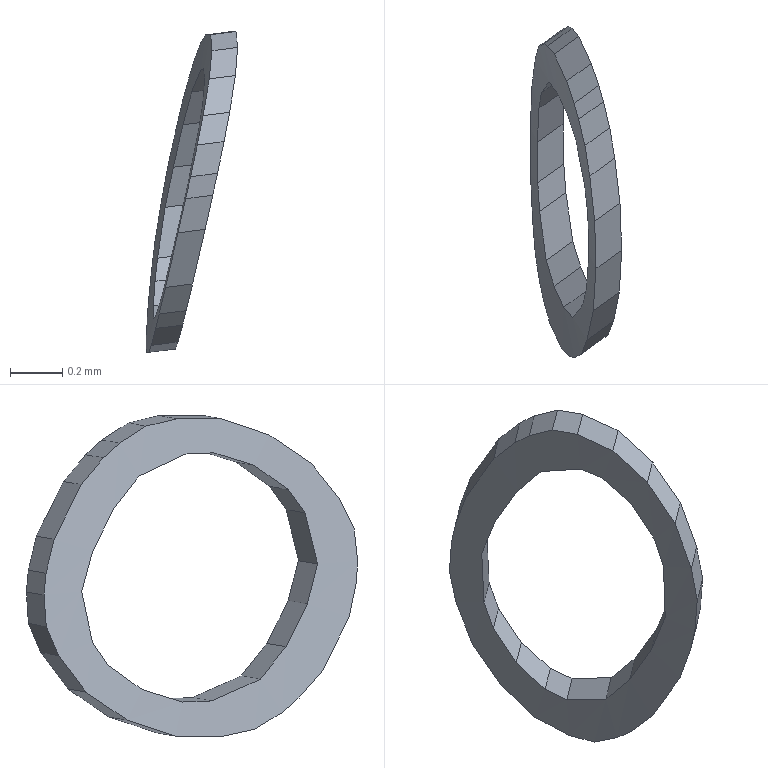Part | SolidWorks | features BaseBody 1 | 1 solid | 46 faces | box 0.3505 x 1.273 x 1.232 mm | volume 0.05013 mm3 | plane 44 | cylinder 2 | commonest cylinder face diameters 16.8 x1 17 x1